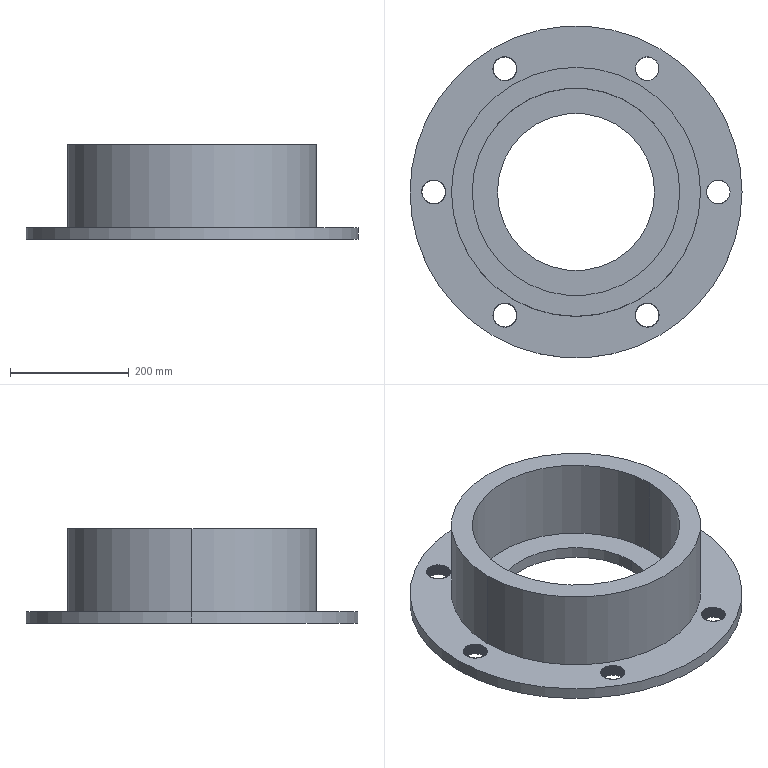Part | SolidWorks | features SweepThread 6, ICE 4, 3DProfileFeature 1, Extrusion 1 | 1 solid | 768 faces | box 560 x 560 x 160 mm | volume 9604413 mm3 | cylinder 734 | spline 18 | plane 16 | commonest cylinder face diameters 40 x726 265 x2 350 x2 420 x2 560 x2